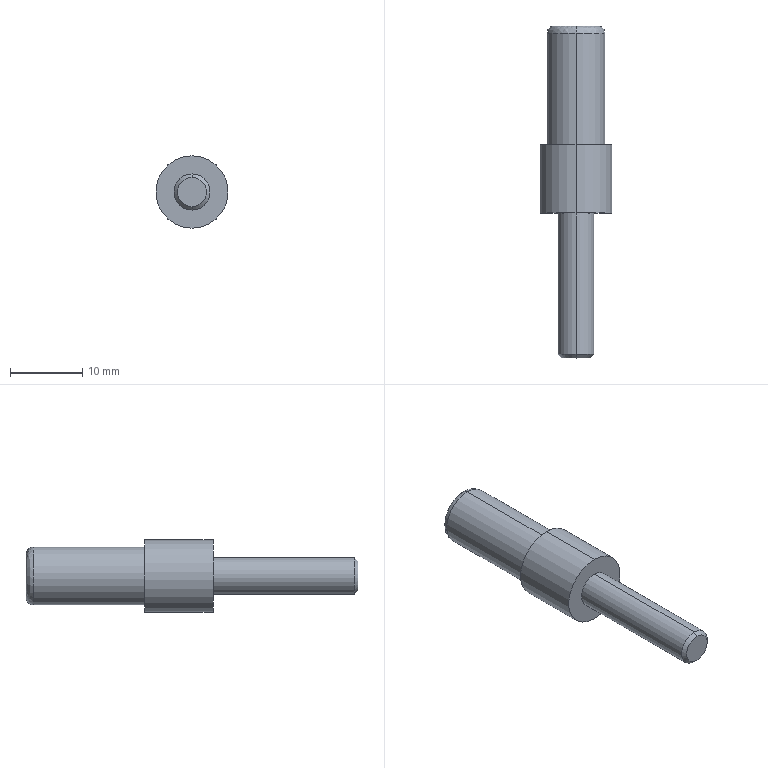Part | STEP file | 0232_Z_CLMS5-20-B_2 | 1 solid | 21 faces | box 10 x 45.8 x 10 mm | volume 1925 mm3 | plane 11 | cylinder 6 | spline 2 | cone 2 | commonest cylinder face diameters 5 x2 8 x2 10 x2